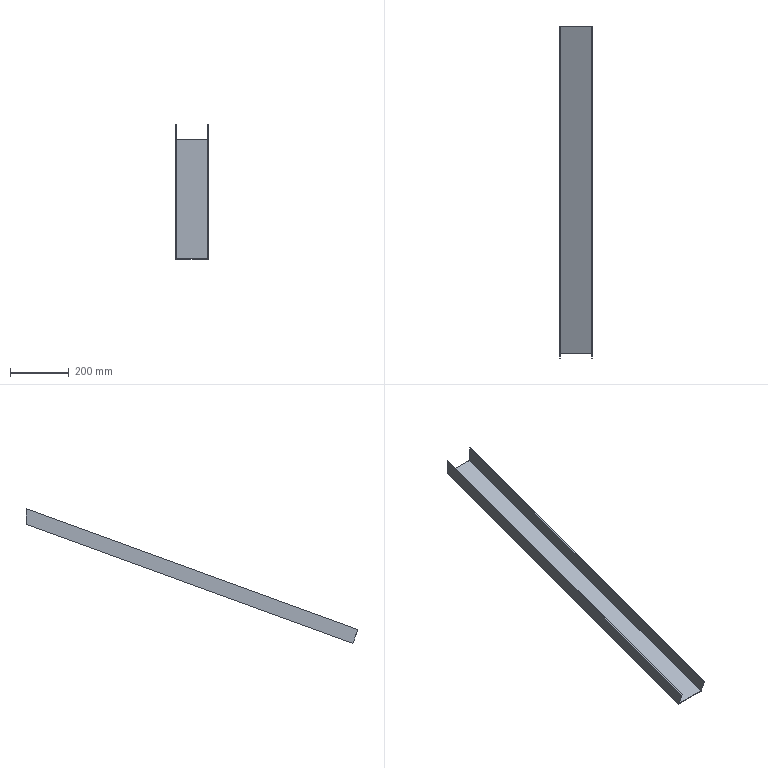Part | NX | features solid 2 | 1 solid | 10 faces | box 110 x 1127 x 457.216 mm | volume 488567 mm3 | plane 10
STEP:
#1=CARTESIAN_POINT('',(45.,85.,-106.054));
#2=VERTEX_POINT('',#1);
#3=CARTESIAN_POINT('',(47.,85.,-106.054));
#4=VERTEX_POINT('',#3);
#5=CARTESIAN_POINT('',(70.,85.,-106.054));
#6=DIRECTION('',(1.,0.,0.));
#7=VECTOR('',#6,1000.);
#8=LINE('',#5,#7);
#9=EDGE_CURVE('',#2,#4,#8,.T.);
#10=ORIENTED_EDGE('',*,*,#9,.T.);
#11=CARTESIAN_POINT('',(47.,85.,-157.135));
#12=VERTEX_POINT('',#11);
#13=CARTESIAN_POINT('',(47.,85.,-335.937));
#14=DIRECTION('',(0.,0.,-1.));
#15=VECTOR('',#14,1000.);
#16=LINE('',#13,#15);
#17=EDGE_CURVE('',#4,#12,#16,.T.);
#18=ORIENTED_EDGE('',*,*,#17,.T.);
#19=CARTESIAN_POINT('',(153.,85.,-157.135));
#20=VERTEX_POINT('',#19);
#21=CARTESIAN_POINT('',(70.,85.,-157.135));
#22=DIRECTION('',(1.,0.,0.));
#23=VECTOR('',#22,1000.);
#24=LINE('',#21,#23);
#25=EDGE_CURVE('',#12,#20,#24,.T.);
#26=ORIENTED_EDGE('',*,*,#25,.T.);
#27=CARTESIAN_POINT('',(153.,85.,-106.054));
#28=VERTEX_POINT('',#27);
#29=CARTESIAN_POINT('',(153.,85.,-80.));
#30=DIRECTION('',(0.,0.,-1.));
#31=VECTOR('',#30,1000.);
#32=LINE('',#29,#31);
#33=EDGE_CURVE('',#28,#20,#32,.T.);
#34=ORIENTED_EDGE('',*,*,#33,.F.);
#35=CARTESIAN_POINT('',(155.,85.,-106.054));
#36=VERTEX_POINT('',#35);
#37=CARTESIAN_POINT('',(70.,85.,-106.054));
#38=DIRECTION('',(1.,0.,0.));
#39=VECTOR('',#38,1000.);
#40=LINE('',#37,#39);
#41=EDGE_CURVE('',#28,#36,#40,.T.);
#42=ORIENTED_EDGE('',*,*,#41,.T.);
#43=CARTESIAN_POINT('',(155.,85.,-159.263));
#44=VERTEX_POINT('',#43);
#45=CARTESIAN_POINT('',(155.,85.,-80.));
#46=DIRECTION('',(0.,0.,-1.));
#47=VECTOR('',#46,1000.);
#48=LINE('',#45,#47);
#49=EDGE_CURVE('',#36,#44,#48,.T.);
#50=ORIENTED_EDGE('',*,*,#49,.T.);
#51=CARTESIAN_POINT('',(45.,85.,-159.263));
#52=VERTEX_POINT('',#51);
#53=CARTESIAN_POINT('',(70.,85.,-159.263));
#54=DIRECTION('',(1.,0.,0.));
#55=VECTOR('',#54,1000.);
#56=LINE('',#53,#55);
#57=EDGE_CURVE('',#52,#44,#56,.T.);
#58=ORIENTED_EDGE('',*,*,#57,.F.);
#59=CARTESIAN_POINT('',(45.,85.,-335.937));
#60=DIRECTION('',(0.,0.,-1.));
#61=VECTOR('',#60,1000.);
#62=LINE('',#59,#61);
#63=EDGE_CURVE('',#2,#52,#62,.T.);
#64=ORIENTED_EDGE('',*,*,#63,.F.);
#65=EDGE_LOOP('',(#10,#18,#26,#34,#42,#50,#58,#64));
#66=FACE_BOUND('',#65,.T.);
#67=CARTESIAN_POINT('',(-855.,85.,-80.));
#68=DIRECTION('',(0.,1.,0.));
#69=DIRECTION('',(-1.,0.,0.));
#70=AXIS2_PLACEMENT_3D('',#67,#68,#69);
#71=PLANE('',#70);
#72=ADVANCED_FACE('',(#66),#71,.T.);
#73=CARTESIAN_POINT('',(155.,-1042.101,-516.286));
#74=VERTEX_POINT('',#73);
#75=CARTESIAN_POINT('',(153.,-1042.101,-516.286));
#76=VERTEX_POINT('',#75);
#77=CARTESIAN_POINT('',(70.,-1042.101,-516.286));
#78=DIRECTION('',(-1.,0.,0.));
#79=VECTOR('',#78,1000.);
#80=LINE('',#77,#79);
#81=EDGE_CURVE('',#74,#76,#80,.T.);
#82=ORIENTED_EDGE('',*,*,#81,.T.);
#83=CARTESIAN_POINT('',(153.,-1025.684,-561.391));
#84=VERTEX_POINT('',#83);
#85=CARTESIAN_POINT('',(153.,-1042.101,-516.286));
#86=DIRECTION('',(0.,0.342,-0.9397));
#87=VECTOR('',#86,1000.);
#88=LINE('',#85,#87);
#89=EDGE_CURVE('',#76,#84,#88,.T.);
#90=ORIENTED_EDGE('',*,*,#89,.T.);
#91=CARTESIAN_POINT('',(47.,-1025.684,-561.391));
#92=VERTEX_POINT('',#91);
#93=CARTESIAN_POINT('',(70.,-1025.684,-561.391));
#94=DIRECTION('',(-1.,0.,0.));
#95=VECTOR('',#94,1000.);
#96=LINE('',#93,#95);
#97=EDGE_CURVE('',#84,#92,#96,.T.);
#98=ORIENTED_EDGE('',*,*,#97,.T.);
#99=CARTESIAN_POINT('',(47.,-1042.101,-516.286));
#100=VERTEX_POINT('',#99);
#101=CARTESIAN_POINT('',(47.,-1042.101,-516.286));
#102=DIRECTION('',(0.,0.342,-0.9397));
#103=VECTOR('',#102,1000.);
#104=LINE('',#101,#103);
#105=EDGE_CURVE('',#100,#92,#104,.T.);
#106=ORIENTED_EDGE('',*,*,#105,.F.);
#107=CARTESIAN_POINT('',(45.,-1042.101,-516.286));
#108=VERTEX_POINT('',#107);
#109=CARTESIAN_POINT('',(70.,-1042.101,-516.286));
#110=DIRECTION('',(-1.,0.,0.));
#111=VECTOR('',#110,1000.);
#112=LINE('',#109,#111);
#113=EDGE_CURVE('',#100,#108,#112,.T.);
#114=ORIENTED_EDGE('',*,*,#113,.T.);
#115=CARTESIAN_POINT('',(45.,-1025.,-563.27));
#116=VERTEX_POINT('',#115);
#117=CARTESIAN_POINT('',(45.,-1042.101,-516.286));
#118=DIRECTION('',(0.,0.342,-0.9397));
#119=VECTOR('',#118,1000.);
#120=LINE('',#117,#119);
#121=EDGE_CURVE('',#108,#116,#120,.T.);
#122=ORIENTED_EDGE('',*,*,#121,.T.);
#123=CARTESIAN_POINT('',(155.,-1025.,-563.27));
#124=VERTEX_POINT('',#123);
#125=CARTESIAN_POINT('',(70.,-1025.,-563.27));
#126=DIRECTION('',(-1.,0.,0.));
#127=VECTOR('',#126,1000.);
#128=LINE('',#125,#127);
#129=EDGE_CURVE('',#124,#116,#128,.T.);
#130=ORIENTED_EDGE('',*,*,#129,.F.);
#131=CARTESIAN_POINT('',(155.,-1042.101,-516.286));
#132=DIRECTION('',(0.,0.342,-0.9397));
#133=VECTOR('',#132,1000.);
#134=LINE('',#131,#133);
#135=EDGE_CURVE('',#74,#124,#134,.T.);
#136=ORIENTED_EDGE('',*,*,#135,.F.);
#137=EDGE_LOOP('',(#82,#90,#98,#106,#114,#122,#130,#136));
#138=FACE_BOUND('',#137,.T.);
#139=CARTESIAN_POINT('',(70.,-1042.101,-516.286));
#140=DIRECTION('',(0.,-0.9397,-0.342));
#141=DIRECTION('',(0.,0.342,-0.9397));
#142=AXIS2_PLACEMENT_3D('',#139,#140,#141);
#143=PLANE('',#142);
#144=ADVANCED_FACE('',(#138),#143,.T.);
#145=ORIENTED_EDGE('',*,*,#113,.F.);
#146=CARTESIAN_POINT('',(47.,-546.597,-335.937));
#147=DIRECTION('',(0.,0.9397,0.342));
#148=VECTOR('',#147,1000.);
#149=LINE('',#146,#148);
#150=EDGE_CURVE('',#100,#4,#149,.T.);
#151=ORIENTED_EDGE('',*,*,#150,.T.);
#152=ORIENTED_EDGE('',*,*,#9,.F.);
#153=CARTESIAN_POINT('',(45.,-546.597,-335.937));
#154=DIRECTION('',(0.,0.9397,0.342));
#155=VECTOR('',#154,1000.);
#156=LINE('',#153,#155);
#157=EDGE_CURVE('',#108,#2,#156,.T.);
#158=ORIENTED_EDGE('',*,*,#157,.F.);
#159=EDGE_LOOP('',(#145,#151,#152,#158));
#160=FACE_BOUND('',#159,.T.);
#161=CARTESIAN_POINT('',(70.,-546.597,-335.937));
#162=DIRECTION('',(0.,0.342,-0.9397));
#163=DIRECTION('',(-1.,0.,0.));
#164=AXIS2_PLACEMENT_3D('',#161,#162,#163);
#165=PLANE('',#164);
#166=ADVANCED_FACE('',(#160),#165,.F.);
#167=CARTESIAN_POINT('',(45.,-529.496,-382.921));
#168=DIRECTION('',(0.,0.9397,0.342));
#169=VECTOR('',#168,1000.);
#170=LINE('',#167,#169);
#171=EDGE_CURVE('',#116,#52,#170,.T.);
#172=ORIENTED_EDGE('',*,*,#171,.F.);
#173=ORIENTED_EDGE('',*,*,#121,.F.);
#174=ORIENTED_EDGE('',*,*,#157,.T.);
#175=ORIENTED_EDGE('',*,*,#63,.T.);
#176=EDGE_LOOP('',(#172,#173,#174,#175));
#177=FACE_BOUND('',#176,.T.);
#178=CARTESIAN_POINT('',(45.,-546.597,-335.937));
#179=DIRECTION('',(-1.,0.,0.));
#180=DIRECTION('',(0.,0.08716,0.9962));
#181=AXIS2_PLACEMENT_3D('',#178,#179,#180);
#182=PLANE('',#181);
#183=ADVANCED_FACE('',(#177),#182,.T.);
#184=CARTESIAN_POINT('',(155.,-529.496,-382.921));
#185=DIRECTION('',(0.,-0.9397,-0.342));
#186=VECTOR('',#185,1000.);
#187=LINE('',#184,#186);
#188=EDGE_CURVE('',#44,#124,#187,.T.);
#189=ORIENTED_EDGE('',*,*,#188,.F.);
#190=ORIENTED_EDGE('',*,*,#49,.F.);
#191=CARTESIAN_POINT('',(155.,-546.597,-335.937));
#192=DIRECTION('',(0.,-0.9397,-0.342));
#193=VECTOR('',#192,1000.);
#194=LINE('',#191,#193);
#195=EDGE_CURVE('',#36,#74,#194,.T.);
#196=ORIENTED_EDGE('',*,*,#195,.T.);
#197=ORIENTED_EDGE('',*,*,#135,.T.);
#198=EDGE_LOOP('',(#189,#190,#196,#197));
#199=FACE_BOUND('',#198,.T.);
#200=CARTESIAN_POINT('',(155.,-546.597,-335.937));
#201=DIRECTION('',(1.,0.,0.));
#202=DIRECTION('',(0.,-0.08716,-0.9962));
#203=AXIS2_PLACEMENT_3D('',#200,#201,#202);
#204=PLANE('',#203);
#205=ADVANCED_FACE('',(#199),#204,.T.);
#206=ORIENTED_EDGE('',*,*,#41,.F.);
#207=CARTESIAN_POINT('',(153.,-546.597,-335.937));
#208=DIRECTION('',(0.,-0.9397,-0.342));
#209=VECTOR('',#208,1000.);
#210=LINE('',#207,#209);
#211=EDGE_CURVE('',#28,#76,#210,.T.);
#212=ORIENTED_EDGE('',*,*,#211,.T.);
#213=ORIENTED_EDGE('',*,*,#81,.F.);
#214=ORIENTED_EDGE('',*,*,#195,.F.);
#215=EDGE_LOOP('',(#206,#212,#213,#214));
#216=FACE_BOUND('',#215,.T.);
#217=CARTESIAN_POINT('',(70.,-546.597,-335.937));
#218=DIRECTION('',(0.,0.342,-0.9397));
#219=DIRECTION('',(-1.,0.,0.));
#220=AXIS2_PLACEMENT_3D('',#217,#218,#219);
#221=PLANE('',#220);
#222=ADVANCED_FACE('',(#216),#221,.F.);
#223=ORIENTED_EDGE('',*,*,#171,.T.);
#224=ORIENTED_EDGE('',*,*,#57,.T.);
#225=ORIENTED_EDGE('',*,*,#188,.T.);
#226=ORIENTED_EDGE('',*,*,#129,.T.);
#227=EDGE_LOOP('',(#223,#224,#225,#226));
#228=FACE_BOUND('',#227,.T.);
#229=CARTESIAN_POINT('',(70.,-529.496,-382.921));
#230=DIRECTION('',(0.,0.342,-0.9397));
#231=DIRECTION('',(-1.,0.,0.));
#232=AXIS2_PLACEMENT_3D('',#229,#230,#231);
#233=PLANE('',#232);
#234=ADVANCED_FACE('',(#228),#233,.T.);
#235=CARTESIAN_POINT('',(47.,-530.18,-381.042));
#236=DIRECTION('',(0.,0.9397,0.342));
#237=VECTOR('',#236,1000.);
#238=LINE('',#235,#237);
#239=EDGE_CURVE('',#92,#12,#238,.T.);
#240=ORIENTED_EDGE('',*,*,#239,.T.);
#241=ORIENTED_EDGE('',*,*,#17,.F.);
#242=ORIENTED_EDGE('',*,*,#150,.F.);
#243=ORIENTED_EDGE('',*,*,#105,.T.);
#244=EDGE_LOOP('',(#240,#241,#242,#243));
#245=FACE_BOUND('',#244,.T.);
#246=CARTESIAN_POINT('',(47.,-546.597,-335.937));
#247=DIRECTION('',(-1.,0.,0.));
#248=DIRECTION('',(0.,0.08716,0.9962));
#249=AXIS2_PLACEMENT_3D('',#246,#247,#248);
#250=PLANE('',#249);
#251=ADVANCED_FACE('',(#245),#250,.F.);
#252=CARTESIAN_POINT('',(153.,-530.18,-381.042));
#253=DIRECTION('',(0.,-0.9397,-0.342));
#254=VECTOR('',#253,1000.);
#255=LINE('',#252,#254);
#256=EDGE_CURVE('',#20,#84,#255,.T.);
#257=ORIENTED_EDGE('',*,*,#256,.T.);
#258=ORIENTED_EDGE('',*,*,#89,.F.);
#259=ORIENTED_EDGE('',*,*,#211,.F.);
#260=ORIENTED_EDGE('',*,*,#33,.T.);
#261=EDGE_LOOP('',(#257,#258,#259,#260));
#262=FACE_BOUND('',#261,.T.);
#263=CARTESIAN_POINT('',(153.,-546.597,-335.937));
#264=DIRECTION('',(1.,0.,0.));
#265=DIRECTION('',(0.,-0.08716,-0.9962));
#266=AXIS2_PLACEMENT_3D('',#263,#264,#265);
#267=PLANE('',#266);
#268=ADVANCED_FACE('',(#262),#267,.F.);
#269=ORIENTED_EDGE('',*,*,#239,.F.);
#270=ORIENTED_EDGE('',*,*,#97,.F.);
#271=ORIENTED_EDGE('',*,*,#256,.F.);
#272=ORIENTED_EDGE('',*,*,#25,.F.);
#273=EDGE_LOOP('',(#269,#270,#271,#272));
#274=FACE_BOUND('',#273,.T.);
#275=CARTESIAN_POINT('',(70.,-530.18,-381.042));
#276=DIRECTION('',(0.,0.342,-0.9397));
#277=DIRECTION('',(-1.,0.,0.));
#278=AXIS2_PLACEMENT_3D('',#275,#276,#277);
#279=PLANE('',#278);
#280=ADVANCED_FACE('',(#274),#279,.F.);
#281=CLOSED_SHELL('',(#72,#144,#166,#183,#205,#222,#234,#251,#268,#280));
#282=MANIFOLD_SOLID_BREP('',#281);
#283=(LENGTH_UNIT()NAMED_UNIT(*)SI_UNIT(.MILLI.,.METRE.));
#284=UNCERTAINTY_MEASURE_WITH_UNIT(LENGTH_MEASURE(0.00001),#283,'','');
#285=(NAMED_UNIT(*)PLANE_ANGLE_UNIT()SI_UNIT($,.RADIAN.));
#286=(NAMED_UNIT(*)SI_UNIT($,.STERADIAN.)SOLID_ANGLE_UNIT());
#287=(GEOMETRIC_REPRESENTATION_CONTEXT(3)GLOBAL_UNCERTAINTY_ASSIGNED_CONTEXT((#284))GLOBAL_UNIT_ASSIGNED_CONTEXT((#283,#285,#286))REPRESENTATION_CONTEXT('',''));
#288=ADVANCED_BREP_SHAPE_REPRESENTATION('',(#282),#287);